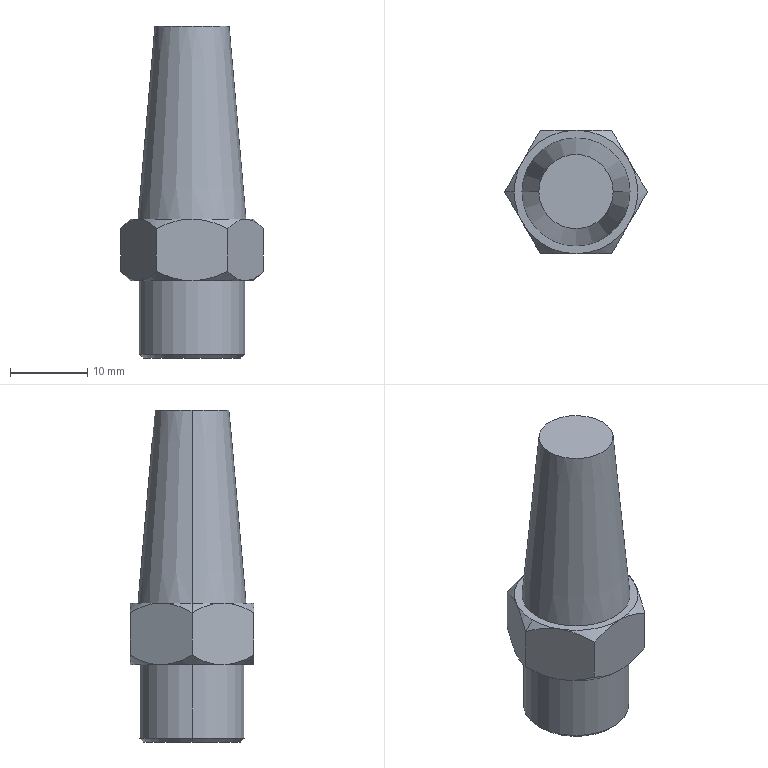Part | SolidWorks | features BaseBody 1 | 1 solid | 33 faces | box 18.475 x 16 x 43 mm | volume 4994 mm3 | cone 18 | plane 11 | cylinder 4 | commonest cylinder face diameters 11.25 x2 13.65 x2
STEP:
#1=CARTESIAN_POINT('',(-4.813,0.,43.));
#2=VERTEX_POINT('',#1);
#3=CARTESIAN_POINT('',(4.813,0.,43.));
#4=VERTEX_POINT('',#3);
#5=CARTESIAN_POINT('',(0.,0.,43.));
#6=DIRECTION('',(0.,0.,-1.));
#7=DIRECTION('',(-1.,0.,0.));
#8=AXIS2_PLACEMENT_3D('',#5,#6,#7);
#9=CIRCLE('',#8,4.813);
#10=EDGE_CURVE('',#2,#4,#9,.T.);
#11=ORIENTED_EDGE('',*,*,#10,.T.);
#12=CARTESIAN_POINT('',(7.,0.,18.));
#13=VERTEX_POINT('',#12);
#14=CARTESIAN_POINT('',(7.,0.,18.));
#15=DIRECTION('',(0.08716,0.,-0.9962));
#16=VECTOR('',#15,1000.);
#17=LINE('',#14,#16);
#18=EDGE_CURVE('',#4,#13,#17,.T.);
#19=ORIENTED_EDGE('',*,*,#18,.T.);
#20=CARTESIAN_POINT('',(-7.,0.,18.));
#21=VERTEX_POINT('',#20);
#22=CARTESIAN_POINT('',(0.,0.,18.));
#23=DIRECTION('',(0.,0.,1.));
#24=DIRECTION('',(-1.,0.,0.));
#25=AXIS2_PLACEMENT_3D('',#22,#23,#24);
#26=CIRCLE('',#25,7.);
#27=EDGE_CURVE('',#13,#21,#26,.T.);
#28=ORIENTED_EDGE('',*,*,#27,.T.);
#29=CARTESIAN_POINT('',(-7.,0.,18.));
#30=DIRECTION('',(-0.08716,0.,-0.9962));
#31=VECTOR('',#30,1000.);
#32=LINE('',#29,#31);
#33=EDGE_CURVE('',#2,#21,#32,.T.);
#34=ORIENTED_EDGE('',*,*,#33,.F.);
#35=EDGE_LOOP('',(#11,#19,#28,#34));
#36=FACE_OUTER_BOUND('',#35,.T.);
#37=CARTESIAN_POINT('',(0.,0.,18.));
#38=DIRECTION('',(0.,0.,-1.));
#39=DIRECTION('',(-1.,0.,0.));
#40=AXIS2_PLACEMENT_3D('',#37,#38,#39);
#41=CONICAL_SURFACE('',#40,7.,0.08727);
#42=ADVANCED_FACE('',(#36),#41,.T.);
#43=CARTESIAN_POINT('',(-8.,0.,18.));
#44=VERTEX_POINT('',#43);
#45=CARTESIAN_POINT('',(-6.928,-4.,18.));
#46=VERTEX_POINT('',#45);
#47=CARTESIAN_POINT('',(0.,0.,18.));
#48=DIRECTION('',(0.,0.,1.));
#49=DIRECTION('',(-1.,0.,0.));
#50=AXIS2_PLACEMENT_3D('',#47,#48,#49);
#51=CIRCLE('',#50,8.);
#52=EDGE_CURVE('',#44,#46,#51,.T.);
#53=ORIENTED_EDGE('',*,*,#52,.F.);
#54=CARTESIAN_POINT('',(-9.238,0.,16.762));
#55=VERTEX_POINT('',#54);
#56=CARTESIAN_POINT('',(-9.245,0.,16.755));
#57=DIRECTION('',(-0.7071,0.,-0.7071));
#58=VECTOR('',#57,1000.);
#59=LINE('',#56,#58);
#60=EDGE_CURVE('',#44,#55,#59,.T.);
#61=ORIENTED_EDGE('',*,*,#60,.T.);
#62=CARTESIAN_POINT('',(-9.238,0.,16.762));
#63=CARTESIAN_POINT('',(-8.876,-0.6269,17.124));
#64=CARTESIAN_POINT('',(-8.506,-1.268,17.432));
#65=CARTESIAN_POINT('',(-7.93,-2.264,17.761));
#66=CARTESIAN_POINT('',(-7.735,-2.602,17.848));
#67=CARTESIAN_POINT('',(-7.337,-3.292,17.968));
#68=CARTESIAN_POINT('',(-7.133,-3.646,18.));
#69=CARTESIAN_POINT('',(-6.928,-4.,18.));
#70=B_SPLINE_CURVE_WITH_KNOTS('',3,(#62,#63,#64,#65,#66,#67,#68,#69),.UNSPECIFIED.,.F.,.F.,(4,2,2,4),(0.,0.002392,0.003589,0.004785),.UNSPECIFIED.);
#71=EDGE_CURVE('',#55,#46,#70,.T.);
#72=ORIENTED_EDGE('',*,*,#71,.T.);
#73=EDGE_LOOP('',(#53,#61,#72));
#74=FACE_OUTER_BOUND('',#73,.T.);
#75=CARTESIAN_POINT('',(0.,0.,16.755));
#76=DIRECTION('',(0.,0.,-1.));
#77=DIRECTION('',(-1.,0.,0.));
#78=AXIS2_PLACEMENT_3D('',#75,#76,#77);
#79=CONICAL_SURFACE('',#78,9.245,0.7854);
#80=ADVANCED_FACE('',(#74),#79,.T.);
#81=CARTESIAN_POINT('',(6.928,-4.,10.));
#82=VERTEX_POINT('',#81);
#83=CARTESIAN_POINT('',(8.,0.,10.));
#84=VERTEX_POINT('',#83);
#85=CARTESIAN_POINT('',(0.,0.,10.));
#86=DIRECTION('',(0.,0.,1.));
#87=DIRECTION('',(1.,0.,0.));
#88=AXIS2_PLACEMENT_3D('',#85,#86,#87);
#89=CIRCLE('',#88,8.);
#90=EDGE_CURVE('',#82,#84,#89,.T.);
#91=ORIENTED_EDGE('',*,*,#90,.T.);
#92=CARTESIAN_POINT('',(9.238,0.,11.238));
#93=VERTEX_POINT('',#92);
#94=CARTESIAN_POINT('',(9.245,0.,11.245));
#95=DIRECTION('',(0.7071,0.,0.7071));
#96=VECTOR('',#95,1000.);
#97=LINE('',#94,#96);
#98=EDGE_CURVE('',#84,#93,#97,.T.);
#99=ORIENTED_EDGE('',*,*,#98,.T.);
#100=CARTESIAN_POINT('',(6.928,-4.,10.));
#101=CARTESIAN_POINT('',(7.334,-3.298,10.));
#102=CARTESIAN_POINT('',(7.728,-2.614,10.125));
#103=CARTESIAN_POINT('',(8.308,-1.61,10.454));
#104=CARTESIAN_POINT('',(8.499,-1.279,10.588));
#105=CARTESIAN_POINT('',(8.874,-0.6306,10.889));
#106=CARTESIAN_POINT('',(9.057,-0.3129,11.057));
#107=CARTESIAN_POINT('',(9.238,0.,11.238));
#108=B_SPLINE_CURVE_WITH_KNOTS('',3,(#100,#101,#102,#103,#104,#105,#106,#107),.UNSPECIFIED.,.F.,.F.,(4,2,2,4),(0.,0.002397,0.003596,0.004794),.UNSPECIFIED.);
#109=EDGE_CURVE('',#82,#93,#108,.T.);
#110=ORIENTED_EDGE('',*,*,#109,.F.);
#111=EDGE_LOOP('',(#91,#99,#110));
#112=FACE_OUTER_BOUND('',#111,.T.);
#113=CARTESIAN_POINT('',(0.,0.,11.245));
#114=DIRECTION('',(0.,0.,1.));
#115=DIRECTION('',(1.,0.,0.));
#116=AXIS2_PLACEMENT_3D('',#113,#114,#115);
#117=CONICAL_SURFACE('',#116,9.245,0.7854);
#118=ADVANCED_FACE('',(#112),#117,.T.);
#119=CARTESIAN_POINT('',(-6.825,0.,10.));
#120=VERTEX_POINT('',#119);
#121=CARTESIAN_POINT('',(6.825,0.,10.));
#122=VERTEX_POINT('',#121);
#123=CARTESIAN_POINT('',(0.,0.,10.));
#124=DIRECTION('',(0.,0.,-1.));
#125=DIRECTION('',(-1.,0.,0.));
#126=AXIS2_PLACEMENT_3D('',#123,#124,#125);
#127=CIRCLE('',#126,6.825);
#128=EDGE_CURVE('',#120,#122,#127,.T.);
#129=ORIENTED_EDGE('',*,*,#128,.T.);
#130=CARTESIAN_POINT('',(6.825,0.,0.5));
#131=VERTEX_POINT('',#130);
#132=CARTESIAN_POINT('',(6.825,0.,10.));
#133=DIRECTION('',(0.,0.,-1.));
#134=VECTOR('',#133,1000.);
#135=LINE('',#132,#134);
#136=EDGE_CURVE('',#122,#131,#135,.T.);
#137=ORIENTED_EDGE('',*,*,#136,.T.);
#138=CARTESIAN_POINT('',(-6.825,0.,0.5));
#139=VERTEX_POINT('',#138);
#140=CARTESIAN_POINT('',(0.,0.,0.5));
#141=DIRECTION('',(0.,0.,1.));
#142=DIRECTION('',(-1.,0.,0.));
#143=AXIS2_PLACEMENT_3D('',#140,#141,#142);
#144=CIRCLE('',#143,6.825);
#145=EDGE_CURVE('',#131,#139,#144,.T.);
#146=ORIENTED_EDGE('',*,*,#145,.T.);
#147=CARTESIAN_POINT('',(-6.825,0.,10.));
#148=DIRECTION('',(0.,0.,-1.));
#149=VECTOR('',#148,1000.);
#150=LINE('',#147,#149);
#151=EDGE_CURVE('',#120,#139,#150,.T.);
#152=ORIENTED_EDGE('',*,*,#151,.F.);
#153=EDGE_LOOP('',(#129,#137,#146,#152));
#154=FACE_OUTER_BOUND('',#153,.T.);
#155=CARTESIAN_POINT('',(0.,0.,10.));
#156=DIRECTION('',(0.,0.,-1.));
#157=DIRECTION('',(-1.,0.,0.));
#158=AXIS2_PLACEMENT_3D('',#155,#156,#157);
#159=CYLINDRICAL_SURFACE('',#158,6.825);
#160=ADVANCED_FACE('',(#154),#159,.T.);
#161=CARTESIAN_POINT('',(6.325,0.,0.));
#162=VERTEX_POINT('',#161);
#163=CARTESIAN_POINT('',(-6.325,0.,0.));
#164=VERTEX_POINT('',#163);
#165=CARTESIAN_POINT('',(0.,0.,0.));
#166=DIRECTION('',(0.,0.,1.));
#167=DIRECTION('',(1.,0.,0.));
#168=AXIS2_PLACEMENT_3D('',#165,#166,#167);
#169=CIRCLE('',#168,6.325);
#170=EDGE_CURVE('',#162,#164,#169,.T.);
#171=ORIENTED_EDGE('',*,*,#170,.T.);
#172=CARTESIAN_POINT('',(-6.825,0.,0.5));
#173=DIRECTION('',(-0.7071,0.,0.7071));
#174=VECTOR('',#173,1000.);
#175=LINE('',#172,#174);
#176=EDGE_CURVE('',#164,#139,#175,.T.);
#177=ORIENTED_EDGE('',*,*,#176,.T.);
#178=ORIENTED_EDGE('',*,*,#145,.F.);
#179=CARTESIAN_POINT('',(6.825,0.,0.5));
#180=DIRECTION('',(0.7071,0.,0.7071));
#181=VECTOR('',#180,1000.);
#182=LINE('',#179,#181);
#183=EDGE_CURVE('',#162,#131,#182,.T.);
#184=ORIENTED_EDGE('',*,*,#183,.F.);
#185=EDGE_LOOP('',(#171,#177,#178,#184));
#186=FACE_OUTER_BOUND('',#185,.T.);
#187=CARTESIAN_POINT('',(0.,0.,0.5));
#188=DIRECTION('',(0.,0.,1.));
#189=DIRECTION('',(1.,0.,0.));
#190=AXIS2_PLACEMENT_3D('',#187,#188,#189);
#191=CONICAL_SURFACE('',#190,6.825,0.7854);
#192=ADVANCED_FACE('',(#186),#191,.T.);
#193=CARTESIAN_POINT('',(5.625,0.,10.));
#194=VERTEX_POINT('',#193);
#195=CARTESIAN_POINT('',(-5.625,0.,10.));
#196=VERTEX_POINT('',#195);
#197=CARTESIAN_POINT('',(0.,0.,10.));
#198=DIRECTION('',(0.,0.,-1.));
#199=DIRECTION('',(-1.,0.,0.));
#200=AXIS2_PLACEMENT_3D('',#197,#198,#199);
#201=CIRCLE('',#200,5.625);
#202=EDGE_CURVE('',#194,#196,#201,.T.);
#203=ORIENTED_EDGE('',*,*,#202,.F.);
#204=CARTESIAN_POINT('',(5.625,0.,0.));
#205=VERTEX_POINT('',#204);
#206=CARTESIAN_POINT('',(5.625,0.,10.));
#207=DIRECTION('',(0.,0.,-1.));
#208=VECTOR('',#207,1000.);
#209=LINE('',#206,#208);
#210=EDGE_CURVE('',#194,#205,#209,.T.);
#211=ORIENTED_EDGE('',*,*,#210,.T.);
#212=CARTESIAN_POINT('',(-5.625,0.,0.));
#213=VERTEX_POINT('',#212);
#214=CARTESIAN_POINT('',(0.,0.,0.));
#215=DIRECTION('',(0.,0.,-1.));
#216=DIRECTION('',(-1.,0.,0.));
#217=AXIS2_PLACEMENT_3D('',#214,#215,#216);
#218=CIRCLE('',#217,5.625);
#219=EDGE_CURVE('',#205,#213,#218,.T.);
#220=ORIENTED_EDGE('',*,*,#219,.T.);
#221=CARTESIAN_POINT('',(-5.625,0.,10.));
#222=DIRECTION('',(0.,0.,-1.));
#223=VECTOR('',#222,1000.);
#224=LINE('',#221,#223);
#225=EDGE_CURVE('',#196,#213,#224,.T.);
#226=ORIENTED_EDGE('',*,*,#225,.F.);
#227=EDGE_LOOP('',(#203,#211,#220,#226));
#228=FACE_OUTER_BOUND('',#227,.T.);
#229=CARTESIAN_POINT('',(0.,0.,10.));
#230=DIRECTION('',(0.,0.,-1.));
#231=DIRECTION('',(-1.,0.,0.));
#232=AXIS2_PLACEMENT_3D('',#229,#230,#231);
#233=CYLINDRICAL_SURFACE('',#232,5.625);
#234=ADVANCED_FACE('',(#228),#233,.F.);
#235=ORIENTED_EDGE('',*,*,#18,.F.);
#236=CARTESIAN_POINT('',(0.,0.,43.));
#237=DIRECTION('',(0.,0.,-1.));
#238=DIRECTION('',(-1.,0.,0.));
#239=AXIS2_PLACEMENT_3D('',#236,#237,#238);
#240=CIRCLE('',#239,4.813);
#241=EDGE_CURVE('',#4,#2,#240,.T.);
#242=ORIENTED_EDGE('',*,*,#241,.T.);
#243=ORIENTED_EDGE('',*,*,#33,.T.);
#244=CARTESIAN_POINT('',(0.,0.,18.));
#245=DIRECTION('',(0.,0.,1.));
#246=DIRECTION('',(-1.,0.,0.));
#247=AXIS2_PLACEMENT_3D('',#244,#245,#246);
#248=CIRCLE('',#247,7.);
#249=EDGE_CURVE('',#21,#13,#248,.T.);
#250=ORIENTED_EDGE('',*,*,#249,.T.);
#251=EDGE_LOOP('',(#235,#242,#243,#250));
#252=FACE_OUTER_BOUND('',#251,.T.);
#253=CARTESIAN_POINT('',(0.,0.,18.));
#254=DIRECTION('',(0.,0.,-1.));
#255=DIRECTION('',(-1.,0.,0.));
#256=AXIS2_PLACEMENT_3D('',#253,#254,#255);
#257=CONICAL_SURFACE('',#256,7.,0.08727);
#258=ADVANCED_FACE('',(#252),#257,.T.);
#259=ORIENTED_EDGE('',*,*,#249,.F.);
#260=ORIENTED_EDGE('',*,*,#27,.F.);
#261=EDGE_LOOP('',(#259,#260));
#262=FACE_BOUND('',#261,.T.);
#263=CARTESIAN_POINT('',(0.,-8.,18.));
#264=VERTEX_POINT('',#263);
#265=CARTESIAN_POINT('',(6.928,-4.,18.));
#266=VERTEX_POINT('',#265);
#267=CARTESIAN_POINT('',(0.,0.,18.));
#268=DIRECTION('',(0.,0.,1.));
#269=DIRECTION('',(-1.,0.,0.));
#270=AXIS2_PLACEMENT_3D('',#267,#268,#269);
#271=CIRCLE('',#270,8.);
#272=EDGE_CURVE('',#264,#266,#271,.T.);
#273=ORIENTED_EDGE('',*,*,#272,.T.);
#274=CARTESIAN_POINT('',(6.928,4.,18.));
#275=VERTEX_POINT('',#274);
#276=CARTESIAN_POINT('',(0.,0.,18.));
#277=DIRECTION('',(0.,0.,1.));
#278=DIRECTION('',(-1.,0.,0.));
#279=AXIS2_PLACEMENT_3D('',#276,#277,#278);
#280=CIRCLE('',#279,8.);
#281=EDGE_CURVE('',#266,#275,#280,.T.);
#282=ORIENTED_EDGE('',*,*,#281,.T.);
#283=CARTESIAN_POINT('',(0.,8.,18.));
#284=VERTEX_POINT('',#283);
#285=CARTESIAN_POINT('',(0.,0.,18.));
#286=DIRECTION('',(0.,0.,1.));
#287=DIRECTION('',(-1.,0.,0.));
#288=AXIS2_PLACEMENT_3D('',#285,#286,#287);
#289=CIRCLE('',#288,8.);
#290=EDGE_CURVE('',#275,#284,#289,.T.);
#291=ORIENTED_EDGE('',*,*,#290,.T.);
#292=CARTESIAN_POINT('',(-6.928,4.,18.));
#293=VERTEX_POINT('',#292);
#294=CARTESIAN_POINT('',(0.,0.,18.));
#295=DIRECTION('',(0.,0.,1.));
#296=DIRECTION('',(-1.,0.,0.));
#297=AXIS2_PLACEMENT_3D('',#294,#295,#296);
#298=CIRCLE('',#297,8.);
#299=EDGE_CURVE('',#284,#293,#298,.T.);
#300=ORIENTED_EDGE('',*,*,#299,.T.);
#301=CARTESIAN_POINT('',(0.,0.,18.));
#302=DIRECTION('',(0.,0.,1.));
#303=DIRECTION('',(-1.,0.,0.));
#304=AXIS2_PLACEMENT_3D('',#301,#302,#303);
#305=CIRCLE('',#304,8.);
#306=EDGE_CURVE('',#293,#44,#305,.T.);
#307=ORIENTED_EDGE('',*,*,#306,.T.);
#308=ORIENTED_EDGE('',*,*,#52,.T.);
#309=CARTESIAN_POINT('',(0.,0.,18.));
#310=DIRECTION('',(0.,0.,1.));
#311=DIRECTION('',(-1.,0.,0.));
#312=AXIS2_PLACEMENT_3D('',#309,#310,#311);
#313=CIRCLE('',#312,8.);
#314=EDGE_CURVE('',#46,#264,#313,.T.);
#315=ORIENTED_EDGE('',*,*,#314,.T.);
#316=EDGE_LOOP('',(#273,#282,#291,#300,#307,#308,#315));
#317=FACE_OUTER_BOUND('',#316,.T.);
#318=CARTESIAN_POINT('',(0.,0.,18.));
#319=DIRECTION('',(0.,0.,1.));
#320=DIRECTION('',(1.,0.,0.));
#321=AXIS2_PLACEMENT_3D('',#318,#319,#320);
#322=PLANE('',#321);
#323=ADVANCED_FACE('',(#262,#317),#322,.T.);
#324=ORIENTED_EDGE('',*,*,#10,.F.);
#325=ORIENTED_EDGE('',*,*,#241,.F.);
#326=EDGE_LOOP('',(#324,#325));
#327=FACE_OUTER_BOUND('',#326,.T.);
#328=CARTESIAN_POINT('',(0.,0.,43.));
#329=DIRECTION('',(0.,0.,1.));
#330=DIRECTION('',(1.,0.,0.));
#331=AXIS2_PLACEMENT_3D('',#328,#329,#330);
#332=PLANE('',#331);
#333=ADVANCED_FACE('',(#327),#332,.T.);
#334=CARTESIAN_POINT('',(9.238,-0.000000006,16.762));
#335=VERTEX_POINT('',#334);
#336=CARTESIAN_POINT('',(6.928,-4.,18.));
#337=CARTESIAN_POINT('',(7.334,-3.298,18.));
#338=CARTESIAN_POINT('',(7.728,-2.614,17.875));
#339=CARTESIAN_POINT('',(8.308,-1.61,17.546));
#340=CARTESIAN_POINT('',(8.499,-1.279,17.412));
#341=CARTESIAN_POINT('',(8.874,-0.6306,17.111));
#342=CARTESIAN_POINT('',(9.057,-0.3129,16.943));
#343=CARTESIAN_POINT('',(9.238,-0.000000006,16.762));
#344=B_SPLINE_CURVE_WITH_KNOTS('',3,(#336,#337,#338,#339,#340,#341,#342,#343),.UNSPECIFIED.,.F.,.F.,(4,2,2,4),(0.,0.002397,0.003596,0.004794),.UNSPECIFIED.);
#345=EDGE_CURVE('',#266,#335,#344,.T.);
#346=ORIENTED_EDGE('',*,*,#345,.T.);
#347=CARTESIAN_POINT('',(9.238,-0.000000006,16.762));
#348=CARTESIAN_POINT('',(8.876,0.6269,17.124));
#349=CARTESIAN_POINT('',(8.506,1.268,17.432));
#350=CARTESIAN_POINT('',(7.93,2.264,17.761));
#351=CARTESIAN_POINT('',(7.735,2.602,17.848));
#352=CARTESIAN_POINT('',(7.337,3.292,17.968));
#353=CARTESIAN_POINT('',(7.133,3.646,18.));
#354=CARTESIAN_POINT('',(6.928,4.,18.));
#355=B_SPLINE_CURVE_WITH_KNOTS('',3,(#347,#348,#349,#350,#351,#352,#353,#354),.UNSPECIFIED.,.F.,.F.,(4,2,2,4),(0.,0.002392,0.003589,0.004785),.UNSPECIFIED.);
#356=EDGE_CURVE('',#335,#275,#355,.T.);
#357=ORIENTED_EDGE('',*,*,#356,.T.);
#358=ORIENTED_EDGE('',*,*,#281,.F.);
#359=EDGE_LOOP('',(#346,#357,#358));
#360=FACE_OUTER_BOUND('',#359,.T.);
#361=CARTESIAN_POINT('',(0.,0.,16.755));
#362=DIRECTION('',(0.,0.,-1.));
#363=DIRECTION('',(-1.,0.,0.));
#364=AXIS2_PLACEMENT_3D('',#361,#362,#363);
#365=CONICAL_SURFACE('',#364,9.245,0.7854);
#366=ADVANCED_FACE('',(#360),#365,.T.);
#367=CARTESIAN_POINT('',(4.619,-8.,16.762));
#368=VERTEX_POINT('',#367);
#369=CARTESIAN_POINT('',(0.,-8.,18.));
#370=CARTESIAN_POINT('',(0.811,-8.,18.));
#371=CARTESIAN_POINT('',(1.6,-8.,17.875));
#372=CARTESIAN_POINT('',(2.76,-8.,17.546));
#373=CARTESIAN_POINT('',(3.142,-8.,17.412));
#374=CARTESIAN_POINT('',(3.891,-8.,17.111));
#375=CARTESIAN_POINT('',(4.257,-8.,16.943));
#376=CARTESIAN_POINT('',(4.619,-8.,16.762));
#377=B_SPLINE_CURVE_WITH_KNOTS('',3,(#369,#370,#371,#372,#373,#374,#375,#376),.UNSPECIFIED.,.F.,.F.,(4,2,2,4),(0.,0.002397,0.003596,0.004794),.UNSPECIFIED.);
#378=EDGE_CURVE('',#264,#368,#377,.T.);
#379=ORIENTED_EDGE('',*,*,#378,.T.);
#380=CARTESIAN_POINT('',(4.619,-8.,16.762));
#381=CARTESIAN_POINT('',(4.981,-7.373,17.124));
#382=CARTESIAN_POINT('',(5.351,-6.732,17.432));
#383=CARTESIAN_POINT('',(5.926,-5.736,17.761));
#384=CARTESIAN_POINT('',(6.121,-5.398,17.848));
#385=CARTESIAN_POINT('',(6.519,-4.708,17.968));
#386=CARTESIAN_POINT('',(6.724,-4.354,18.));
#387=CARTESIAN_POINT('',(6.928,-4.,18.));
#388=B_SPLINE_CURVE_WITH_KNOTS('',3,(#380,#381,#382,#383,#384,#385,#386,#387),.UNSPECIFIED.,.F.,.F.,(4,2,2,4),(0.,0.002392,0.003589,0.004785),.UNSPECIFIED.);
#389=EDGE_CURVE('',#368,#266,#388,.T.);
#390=ORIENTED_EDGE('',*,*,#389,.T.);
#391=ORIENTED_EDGE('',*,*,#272,.F.);
#392=EDGE_LOOP('',(#379,#390,#391));
#393=FACE_OUTER_BOUND('',#392,.T.);
#394=CARTESIAN_POINT('',(0.,0.,16.755));
#395=DIRECTION('',(0.,0.,-1.));
#396=DIRECTION('',(-1.,0.,0.));
#397=AXIS2_PLACEMENT_3D('',#394,#395,#396);
#398=CONICAL_SURFACE('',#397,9.245,0.7854);
#399=ADVANCED_FACE('',(#393),#398,.T.);
#400=CARTESIAN_POINT('',(-4.619,-8.,16.762));
#401=VERTEX_POINT('',#400);
#402=CARTESIAN_POINT('',(-6.928,-4.,18.));
#403=CARTESIAN_POINT('',(-6.523,-4.702,18.));
#404=CARTESIAN_POINT('',(-6.128,-5.386,17.875));
#405=CARTESIAN_POINT('',(-5.548,-6.39,17.546));
#406=CARTESIAN_POINT('',(-5.357,-6.721,17.412));
#407=CARTESIAN_POINT('',(-4.983,-7.369,17.111));
#408=CARTESIAN_POINT('',(-4.799,-7.687,16.943));
#409=CARTESIAN_POINT('',(-4.619,-8.,16.762));
#410=B_SPLINE_CURVE_WITH_KNOTS('',3,(#402,#403,#404,#405,#406,#407,#408,#409),.UNSPECIFIED.,.F.,.F.,(4,2,2,4),(0.,0.002397,0.003596,0.004794),.UNSPECIFIED.);
#411=EDGE_CURVE('',#46,#401,#410,.T.);
#412=ORIENTED_EDGE('',*,*,#411,.T.);
#413=CARTESIAN_POINT('',(-4.619,-8.,16.762));
#414=CARTESIAN_POINT('',(-3.895,-8.,17.124));
#415=CARTESIAN_POINT('',(-3.155,-8.,17.432));
#416=CARTESIAN_POINT('',(-2.005,-8.,17.761));
#417=CARTESIAN_POINT('',(-1.614,-8.,17.848));
#418=CARTESIAN_POINT('',(-0.8177,-8.,17.968));
#419=CARTESIAN_POINT('',(-0.4086,-8.,18.));
#420=CARTESIAN_POINT('',(0.,-8.,18.));
#421=B_SPLINE_CURVE_WITH_KNOTS('',3,(#413,#414,#415,#416,#417,#418,#419,#420),.UNSPECIFIED.,.F.,.F.,(4,2,2,4),(0.,0.002392,0.003589,0.004785),.UNSPECIFIED.);
#422=EDGE_CURVE('',#401,#264,#421,.T.);
#423=ORIENTED_EDGE('',*,*,#422,.T.);
#424=ORIENTED_EDGE('',*,*,#314,.F.);
#425=EDGE_LOOP('',(#412,#423,#424));
#426=FACE_OUTER_BOUND('',#425,.T.);
#427=CARTESIAN_POINT('',(0.,0.,16.755));
#428=DIRECTION('',(0.,0.,-1.));
#429=DIRECTION('',(-1.,0.,0.));
#430=AXIS2_PLACEMENT_3D('',#427,#428,#429);
#431=CONICAL_SURFACE('',#430,9.245,0.7854);
#432=ADVANCED_FACE('',(#426),#431,.T.);
#433=ORIENTED_EDGE('',*,*,#60,.F.);
#434=ORIENTED_EDGE('',*,*,#306,.F.);
#435=CARTESIAN_POINT('',(-6.928,4.,18.));
#436=CARTESIAN_POINT('',(-7.334,3.298,18.));
#437=CARTESIAN_POINT('',(-7.728,2.614,17.875));
#438=CARTESIAN_POINT('',(-8.308,1.61,17.546));
#439=CARTESIAN_POINT('',(-8.499,1.279,17.412));
#440=CARTESIAN_POINT('',(-8.874,0.6306,17.111));
#441=CARTESIAN_POINT('',(-9.057,0.3129,16.943));
#442=CARTESIAN_POINT('',(-9.238,0.,16.762));
#443=B_SPLINE_CURVE_WITH_KNOTS('',3,(#435,#436,#437,#438,#439,#440,#441,#442),.UNSPECIFIED.,.F.,.F.,(4,2,2,4),(0.,0.002397,0.003596,0.004794),.UNSPECIFIED.);
#444=EDGE_CURVE('',#293,#55,#443,.T.);
#445=ORIENTED_EDGE('',*,*,#444,.T.);
#446=EDGE_LOOP('',(#433,#434,#445));
#447=FACE_OUTER_BOUND('',#446,.T.);
#448=CARTESIAN_POINT('',(0.,0.,16.755));
#449=DIRECTION('',(0.,0.,-1.));
#450=DIRECTION('',(-1.,0.,0.));
#451=AXIS2_PLACEMENT_3D('',#448,#449,#450);
#452=CONICAL_SURFACE('',#451,9.245,0.7854);
#453=ADVANCED_FACE('',(#447),#452,.T.);
#454=CARTESIAN_POINT('',(-4.619,8.,16.762));
#455=VERTEX_POINT('',#454);
#456=CARTESIAN_POINT('',(-4.619,8.,16.762));
#457=CARTESIAN_POINT('',(-4.981,7.373,17.124));
#458=CARTESIAN_POINT('',(-5.351,6.732,17.432));
#459=CARTESIAN_POINT('',(-5.926,5.736,17.761));
#460=CARTESIAN_POINT('',(-6.121,5.398,17.848));
#461=CARTESIAN_POINT('',(-6.519,4.708,17.968));
#462=CARTESIAN_POINT('',(-6.724,4.354,18.));
#463=CARTESIAN_POINT('',(-6.928,4.,18.));
#464=B_SPLINE_CURVE_WITH_KNOTS('',3,(#456,#457,#458,#459,#460,#461,#462,#463),.UNSPECIFIED.,.F.,.F.,(4,2,2,4),(0.,0.002392,0.003589,0.004785),.UNSPECIFIED.);
#465=EDGE_CURVE('',#455,#293,#464,.T.);
#466=ORIENTED_EDGE('',*,*,#465,.T.);
#467=ORIENTED_EDGE('',*,*,#299,.F.);
#468=CARTESIAN_POINT('',(0.,8.,18.));
#469=CARTESIAN_POINT('',(-0.811,8.,18.));
#470=CARTESIAN_POINT('',(-1.6,8.,17.875));
#471=CARTESIAN_POINT('',(-2.76,8.,17.546));
#472=CARTESIAN_POINT('',(-3.142,8.,17.412));
#473=CARTESIAN_POINT('',(-3.891,8.,17.111));
#474=CARTESIAN_POINT('',(-4.257,8.,16.943));
#475=CARTESIAN_POINT('',(-4.619,8.,16.762));
#476=B_SPLINE_CURVE_WITH_KNOTS('',3,(#468,#469,#470,#471,#472,#473,#474,#475),.UNSPECIFIED.,.F.,.F.,(4,2,2,4),(0.,0.002397,0.003596,0.004794),.UNSPECIFIED.);
#477=EDGE_CURVE('',#284,#455,#476,.T.);
#478=ORIENTED_EDGE('',*,*,#477,.T.);
#479=EDGE_LOOP('',(#466,#467,#478));
#480=FACE_OUTER_BOUND('',#479,.T.);
#481=CARTESIAN_POINT('',(0.,0.,16.755));
#482=DIRECTION('',(0.,0.,-1.));
#483=DIRECTION('',(-1.,0.,0.));
#484=AXIS2_PLACEMENT_3D('',#481,#482,#483);
#485=CONICAL_SURFACE('',#484,9.245,0.7854);
#486=ADVANCED_FACE('',(#480),#485,.T.);
#487=CARTESIAN_POINT('',(4.619,8.,16.762));
#488=VERTEX_POINT('',#487);
#489=CARTESIAN_POINT('',(4.619,8.,16.762));
#490=CARTESIAN_POINT('',(3.895,8.,17.124));
#491=CARTESIAN_POINT('',(3.155,8.,17.432));
#492=CARTESIAN_POINT('',(2.005,8.,17.761));
#493=CARTESIAN_POINT('',(1.614,8.,17.848));
#494=CARTESIAN_POINT('',(0.8177,8.,17.968));
#495=CARTESIAN_POINT('',(0.4086,8.,18.));
#496=CARTESIAN_POINT('',(0.,8.,18.));
#497=B_SPLINE_CURVE_WITH_KNOTS('',3,(#489,#490,#491,#492,#493,#494,#495,#496),.UNSPECIFIED.,.F.,.F.,(4,2,2,4),(0.,0.002392,0.003589,0.004785),.UNSPECIFIED.);
#498=EDGE_CURVE('',#488,#284,#497,.T.);
#499=ORIENTED_EDGE('',*,*,#498,.T.);
#500=ORIENTED_EDGE('',*,*,#290,.F.);
#501=CARTESIAN_POINT('',(6.928,4.,18.));
#502=CARTESIAN_POINT('',(6.523,4.702,18.));
#503=CARTESIAN_POINT('',(6.128,5.386,17.875));
#504=CARTESIAN_POINT('',(5.548,6.39,17.546));
#505=CARTESIAN_POINT('',(5.357,6.721,17.412));
#506=CARTESIAN_POINT('',(4.983,7.369,17.111));
#507=CARTESIAN_POINT('',(4.799,7.687,16.943));
#508=CARTESIAN_POINT('',(4.619,8.,16.762));
#509=B_SPLINE_CURVE_WITH_KNOTS('',3,(#501,#502,#503,#504,#505,#506,#507,#508),.UNSPECIFIED.,.F.,.F.,(4,2,2,4),(0.,0.002397,0.003596,0.004794),.UNSPECIFIED.);
#510=EDGE_CURVE('',#275,#488,#509,.T.);
#511=ORIENTED_EDGE('',*,*,#510,.T.);
#512=EDGE_LOOP('',(#499,#500,#511));
#513=FACE_OUTER_BOUND('',#512,.T.);
#514=CARTESIAN_POINT('',(0.,0.,16.755));
#515=DIRECTION('',(0.,0.,-1.));
#516=DIRECTION('',(-1.,0.,0.));
#517=AXIS2_PLACEMENT_3D('',#514,#515,#516);
#518=CONICAL_SURFACE('',#517,9.245,0.7854);
#519=ADVANCED_FACE('',(#513),#518,.T.);
#520=CARTESIAN_POINT('',(6.928,4.,10.));
#521=VERTEX_POINT('',#520);
#522=CARTESIAN_POINT('',(9.238,0.,11.238));
#523=CARTESIAN_POINT('',(8.876,0.6269,10.876));
#524=CARTESIAN_POINT('',(8.506,1.268,10.568));
#525=CARTESIAN_POINT('',(7.93,2.264,10.239));
#526=CARTESIAN_POINT('',(7.735,2.602,10.152));
#527=CARTESIAN_POINT('',(7.337,3.292,10.032));
#528=CARTESIAN_POINT('',(7.133,3.646,10.));
#529=CARTESIAN_POINT('',(6.928,4.,10.));
#530=B_SPLINE_CURVE_WITH_KNOTS('',3,(#522,#523,#524,#525,#526,#527,#528,#529),.UNSPECIFIED.,.F.,.F.,(4,2,2,4),(0.,0.002392,0.003589,0.004785),.UNSPECIFIED.);
#531=EDGE_CURVE('',#93,#521,#530,.T.);
#532=ORIENTED_EDGE('',*,*,#531,.T.);
#533=CARTESIAN_POINT('',(4.619,8.,11.238));
#534=VERTEX_POINT('',#533);
#535=CARTESIAN_POINT('',(6.928,4.,10.));
#536=CARTESIAN_POINT('',(6.523,4.702,10.));
#537=CARTESIAN_POINT('',(6.128,5.386,10.125));
#538=CARTESIAN_POINT('',(5.548,6.39,10.454));
#539=CARTESIAN_POINT('',(5.357,6.721,10.588));
#540=CARTESIAN_POINT('',(4.983,7.369,10.889));
#541=CARTESIAN_POINT('',(4.799,7.687,11.057));
#542=CARTESIAN_POINT('',(4.619,8.,11.238));
#543=B_SPLINE_CURVE_WITH_KNOTS('',3,(#535,#536,#537,#538,#539,#540,#541,#542),.UNSPECIFIED.,.F.,.F.,(4,2,2,4),(0.,0.002397,0.003596,0.004794),.UNSPECIFIED.);
#544=EDGE_CURVE('',#521,#534,#543,.T.);
#545=ORIENTED_EDGE('',*,*,#544,.T.);
#546=CARTESIAN_POINT('',(4.619,8.,10.));
#547=DIRECTION('',(0.,0.,1.));
#548=VECTOR('',#547,1000.);
#549=LINE('',#546,#548);
#550=EDGE_CURVE('',#534,#488,#549,.T.);
#551=ORIENTED_EDGE('',*,*,#550,.T.);
#552=ORIENTED_EDGE('',*,*,#510,.F.);
#553=ORIENTED_EDGE('',*,*,#356,.F.);
#554=CARTESIAN_POINT('',(9.238,0.,10.));
#555=DIRECTION('',(0.,0.,-1.));
#556=VECTOR('',#555,1000.);
#557=LINE('',#554,#556);
#558=EDGE_CURVE('',#335,#93,#557,.T.);
#559=ORIENTED_EDGE('',*,*,#558,.T.);
#560=EDGE_LOOP('',(#532,#545,#551,#552,#553,#559));
#561=FACE_OUTER_BOUND('',#560,.T.);
#562=CARTESIAN_POINT('',(9.238,0.,10.));
#563=DIRECTION('',(0.866,0.5,0.));
#564=DIRECTION('',(-0.5,0.866,0.));
#565=AXIS2_PLACEMENT_3D('',#562,#563,#564);
#566=PLANE('',#565);
#567=ADVANCED_FACE('',(#561),#566,.T.);
#568=CARTESIAN_POINT('',(4.619,-8.,11.238));
#569=VERTEX_POINT('',#568);
#570=CARTESIAN_POINT('',(4.619,-8.,11.238));
#571=CARTESIAN_POINT('',(4.981,-7.373,10.876));
#572=CARTESIAN_POINT('',(5.351,-6.732,10.568));
#573=CARTESIAN_POINT('',(5.926,-5.736,10.239));
#574=CARTESIAN_POINT('',(6.121,-5.398,10.152));
#575=CARTESIAN_POINT('',(6.519,-4.708,10.032));
#576=CARTESIAN_POINT('',(6.724,-4.354,10.));
#577=CARTESIAN_POINT('',(6.928,-4.,10.));
#578=B_SPLINE_CURVE_WITH_KNOTS('',3,(#570,#571,#572,#573,#574,#575,#576,#577),.UNSPECIFIED.,.F.,.F.,(4,2,2,4),(0.,0.002392,0.003589,0.004785),.UNSPECIFIED.);
#579=EDGE_CURVE('',#569,#82,#578,.T.);
#580=ORIENTED_EDGE('',*,*,#579,.T.);
#581=ORIENTED_EDGE('',*,*,#109,.T.);
#582=ORIENTED_EDGE('',*,*,#558,.F.);
#583=ORIENTED_EDGE('',*,*,#345,.F.);
#584=ORIENTED_EDGE('',*,*,#389,.F.);
#585=CARTESIAN_POINT('',(4.619,-8.,10.));
#586=DIRECTION('',(0.,0.,-1.));
#587=VECTOR('',#586,1000.);
#588=LINE('',#585,#587);
#589=EDGE_CURVE('',#368,#569,#588,.T.);
#590=ORIENTED_EDGE('',*,*,#589,.T.);
#591=EDGE_LOOP('',(#580,#581,#582,#583,#584,#590));
#592=FACE_OUTER_BOUND('',#591,.T.);
#593=CARTESIAN_POINT('',(4.619,-8.,10.));
#594=DIRECTION('',(0.866,-0.5,0.));
#595=DIRECTION('',(0.5,0.866,0.));
#596=AXIS2_PLACEMENT_3D('',#593,#594,#595);
#597=PLANE('',#596);
#598=ADVANCED_FACE('',(#592),#597,.T.);
#599=CARTESIAN_POINT('',(-4.619,-8.,11.238));
#600=VERTEX_POINT('',#599);
#601=CARTESIAN_POINT('',(0.,-8.,10.));
#602=VERTEX_POINT('',#601);
#603=CARTESIAN_POINT('',(-4.619,-8.,11.238));
#604=CARTESIAN_POINT('',(-3.895,-8.,10.876));
#605=CARTESIAN_POINT('',(-3.155,-8.,10.568));
#606=CARTESIAN_POINT('',(-2.005,-8.,10.239));
#607=CARTESIAN_POINT('',(-1.614,-8.,10.152));
#608=CARTESIAN_POINT('',(-0.8177,-8.,10.032));
#609=CARTESIAN_POINT('',(-0.4086,-8.,10.));
#610=CARTESIAN_POINT('',(0.,-8.,10.));
#611=B_SPLINE_CURVE_WITH_KNOTS('',3,(#603,#604,#605,#606,#607,#608,#609,#610),.UNSPECIFIED.,.F.,.F.,(4,2,2,4),(0.,0.002392,0.003589,0.004785),.UNSPECIFIED.);
#612=EDGE_CURVE('',#600,#602,#611,.T.);
#613=ORIENTED_EDGE('',*,*,#612,.T.);
#614=CARTESIAN_POINT('',(0.,-8.,10.));
#615=CARTESIAN_POINT('',(0.811,-8.,10.));
#616=CARTESIAN_POINT('',(1.6,-8.,10.125));
#617=CARTESIAN_POINT('',(2.76,-8.,10.454));
#618=CARTESIAN_POINT('',(3.142,-8.,10.588));
#619=CARTESIAN_POINT('',(3.891,-8.,10.889));
#620=CARTESIAN_POINT('',(4.257,-8.,11.057));
#621=CARTESIAN_POINT('',(4.619,-8.,11.238));
#622=B_SPLINE_CURVE_WITH_KNOTS('',3,(#614,#615,#616,#617,#618,#619,#620,#621),.UNSPECIFIED.,.F.,.F.,(4,2,2,4),(0.,0.002397,0.003596,0.004794),.UNSPECIFIED.);
#623=EDGE_CURVE('',#602,#569,#622,.T.);
#624=ORIENTED_EDGE('',*,*,#623,.T.);
#625=ORIENTED_EDGE('',*,*,#589,.F.);
#626=ORIENTED_EDGE('',*,*,#378,.F.);
#627=ORIENTED_EDGE('',*,*,#422,.F.);
#628=CARTESIAN_POINT('',(-4.619,-8.,10.));
#629=DIRECTION('',(0.,0.,-1.));
#630=VECTOR('',#629,1000.);
#631=LINE('',#628,#630);
#632=EDGE_CURVE('',#401,#600,#631,.T.);
#633=ORIENTED_EDGE('',*,*,#632,.T.);
#634=EDGE_LOOP('',(#613,#624,#625,#626,#627,#633));
#635=FACE_OUTER_BOUND('',#634,.T.);
#636=CARTESIAN_POINT('',(-4.619,-8.,10.));
#637=DIRECTION('',(0.,-1.,0.));
#638=DIRECTION('',(1.,0.,0.));
#639=AXIS2_PLACEMENT_3D('',#636,#637,#638);
#640=PLANE('',#639);
#641=ADVANCED_FACE('',(#635),#640,.T.);
#642=CARTESIAN_POINT('',(-9.238,0.,11.238));
#643=VERTEX_POINT('',#642);
#644=CARTESIAN_POINT('',(-6.928,-4.,10.));
#645=VERTEX_POINT('',#644);
#646=CARTESIAN_POINT('',(-9.238,0.,11.238));
#647=CARTESIAN_POINT('',(-8.876,-0.6269,10.876));
#648=CARTESIAN_POINT('',(-8.506,-1.268,10.568));
#649=CARTESIAN_POINT('',(-7.93,-2.264,10.239));
#650=CARTESIAN_POINT('',(-7.735,-2.602,10.152));
#651=CARTESIAN_POINT('',(-7.337,-3.292,10.032));
#652=CARTESIAN_POINT('',(-7.133,-3.646,10.));
#653=CARTESIAN_POINT('',(-6.928,-4.,10.));
#654=B_SPLINE_CURVE_WITH_KNOTS('',3,(#646,#647,#648,#649,#650,#651,#652,#653),.UNSPECIFIED.,.F.,.F.,(4,2,2,4),(0.,0.002392,0.003589,0.004785),.UNSPECIFIED.);
#655=EDGE_CURVE('',#643,#645,#654,.T.);
#656=ORIENTED_EDGE('',*,*,#655,.T.);
#657=CARTESIAN_POINT('',(-6.928,-4.,10.));
#658=CARTESIAN_POINT('',(-6.523,-4.702,10.));
#659=CARTESIAN_POINT('',(-6.128,-5.386,10.125));
#660=CARTESIAN_POINT('',(-5.548,-6.39,10.454));
#661=CARTESIAN_POINT('',(-5.357,-6.721,10.588));
#662=CARTESIAN_POINT('',(-4.983,-7.369,10.889));
#663=CARTESIAN_POINT('',(-4.799,-7.687,11.057));
#664=CARTESIAN_POINT('',(-4.619,-8.,11.238));
#665=B_SPLINE_CURVE_WITH_KNOTS('',3,(#657,#658,#659,#660,#661,#662,#663,#664),.UNSPECIFIED.,.F.,.F.,(4,2,2,4),(0.,0.002397,0.003596,0.004794),.UNSPECIFIED.);
#666=EDGE_CURVE('',#645,#600,#665,.T.);
#667=ORIENTED_EDGE('',*,*,#666,.T.);
#668=ORIENTED_EDGE('',*,*,#632,.F.);
#669=ORIENTED_EDGE('',*,*,#411,.F.);
#670=ORIENTED_EDGE('',*,*,#71,.F.);
#671=CARTESIAN_POINT('',(-9.238,0.,10.));
#672=DIRECTION('',(0.,0.,-1.));
#673=VECTOR('',#672,1000.);
#674=LINE('',#671,#673);
#675=EDGE_CURVE('',#55,#643,#674,.T.);
#676=ORIENTED_EDGE('',*,*,#675,.T.);
#677=EDGE_LOOP('',(#656,#667,#668,#669,#670,#676));
#678=FACE_OUTER_BOUND('',#677,.T.);
#679=CARTESIAN_POINT('',(-9.238,0.,10.));
#680=DIRECTION('',(-0.866,-0.5,0.));
#681=DIRECTION('',(0.5,-0.866,0.));
#682=AXIS2_PLACEMENT_3D('',#679,#680,#681);
#683=PLANE('',#682);
#684=ADVANCED_FACE('',(#678),#683,.T.);
#685=CARTESIAN_POINT('',(-4.619,8.,11.238));
#686=VERTEX_POINT('',#685);
#687=CARTESIAN_POINT('',(-6.928,4.,10.));
#688=VERTEX_POINT('',#687);
#689=CARTESIAN_POINT('',(-4.619,8.,11.238));
#690=CARTESIAN_POINT('',(-4.981,7.373,10.876));
#691=CARTESIAN_POINT('',(-5.351,6.732,10.568));
#692=CARTESIAN_POINT('',(-5.926,5.736,10.239));
#693=CARTESIAN_POINT('',(-6.121,5.398,10.152));
#694=CARTESIAN_POINT('',(-6.519,4.708,10.032));
#695=CARTESIAN_POINT('',(-6.724,4.354,10.));
#696=CARTESIAN_POINT('',(-6.928,4.,10.));
#697=B_SPLINE_CURVE_WITH_KNOTS('',3,(#689,#690,#691,#692,#693,#694,#695,#696),.UNSPECIFIED.,.F.,.F.,(4,2,2,4),(0.,0.002392,0.003589,0.004785),.UNSPECIFIED.);
#698=EDGE_CURVE('',#686,#688,#697,.T.);
#699=ORIENTED_EDGE('',*,*,#698,.T.);
#700=CARTESIAN_POINT('',(-6.928,4.,10.));
#701=CARTESIAN_POINT('',(-7.334,3.298,10.));
#702=CARTESIAN_POINT('',(-7.728,2.614,10.125));
#703=CARTESIAN_POINT('',(-8.308,1.61,10.454));
#704=CARTESIAN_POINT('',(-8.499,1.279,10.588));
#705=CARTESIAN_POINT('',(-8.874,0.6306,10.889));
#706=CARTESIAN_POINT('',(-9.057,0.3129,11.057));
#707=CARTESIAN_POINT('',(-9.238,0.,11.238));
#708=B_SPLINE_CURVE_WITH_KNOTS('',3,(#700,#701,#702,#703,#704,#705,#706,#707),.UNSPECIFIED.,.F.,.F.,(4,2,2,4),(0.,0.002397,0.003596,0.004794),.UNSPECIFIED.);
#709=EDGE_CURVE('',#688,#643,#708,.T.);
#710=ORIENTED_EDGE('',*,*,#709,.T.);
#711=ORIENTED_EDGE('',*,*,#675,.F.);
#712=ORIENTED_EDGE('',*,*,#444,.F.);
#713=ORIENTED_EDGE('',*,*,#465,.F.);
#714=CARTESIAN_POINT('',(-4.619,8.,10.));
#715=DIRECTION('',(0.,0.,-1.));
#716=VECTOR('',#715,1000.);
#717=LINE('',#714,#716);
#718=EDGE_CURVE('',#455,#686,#717,.T.);
#719=ORIENTED_EDGE('',*,*,#718,.T.);
#720=EDGE_LOOP('',(#699,#710,#711,#712,#713,#719));
#721=FACE_OUTER_BOUND('',#720,.T.);
#722=CARTESIAN_POINT('',(-4.619,8.,10.));
#723=DIRECTION('',(-0.866,0.5,0.));
#724=DIRECTION('',(-0.5,-0.866,0.));
#725=AXIS2_PLACEMENT_3D('',#722,#723,#724);
#726=PLANE('',#725);
#727=ADVANCED_FACE('',(#721),#726,.T.);
#728=CARTESIAN_POINT('',(0.,8.,10.));
#729=VERTEX_POINT('',#728);
#730=CARTESIAN_POINT('',(4.619,8.,11.238));
#731=CARTESIAN_POINT('',(3.895,8.,10.876));
#732=CARTESIAN_POINT('',(3.155,8.,10.568));
#733=CARTESIAN_POINT('',(2.005,8.,10.239));
#734=CARTESIAN_POINT('',(1.614,8.,10.152));
#735=CARTESIAN_POINT('',(0.8177,8.,10.032));
#736=CARTESIAN_POINT('',(0.4086,8.,10.));
#737=CARTESIAN_POINT('',(0.,8.,10.));
#738=B_SPLINE_CURVE_WITH_KNOTS('',3,(#730,#731,#732,#733,#734,#735,#736,#737),.UNSPECIFIED.,.F.,.F.,(4,2,2,4),(0.,0.002392,0.003589,0.004785),.UNSPECIFIED.);
#739=EDGE_CURVE('',#534,#729,#738,.T.);
#740=ORIENTED_EDGE('',*,*,#739,.T.);
#741=CARTESIAN_POINT('',(0.,8.,10.));
#742=CARTESIAN_POINT('',(-0.811,8.,10.));
#743=CARTESIAN_POINT('',(-1.6,8.,10.125));
#744=CARTESIAN_POINT('',(-2.76,8.,10.454));
#745=CARTESIAN_POINT('',(-3.142,8.,10.588));
#746=CARTESIAN_POINT('',(-3.891,8.,10.889));
#747=CARTESIAN_POINT('',(-4.257,8.,11.057));
#748=CARTESIAN_POINT('',(-4.619,8.,11.238));
#749=B_SPLINE_CURVE_WITH_KNOTS('',3,(#741,#742,#743,#744,#745,#746,#747,#748),.UNSPECIFIED.,.F.,.F.,(4,2,2,4),(0.,0.002397,0.003596,0.004794),.UNSPECIFIED.);
#750=EDGE_CURVE('',#729,#686,#749,.T.);
#751=ORIENTED_EDGE('',*,*,#750,.T.);
#752=ORIENTED_EDGE('',*,*,#718,.F.);
#753=ORIENTED_EDGE('',*,*,#477,.F.);
#754=ORIENTED_EDGE('',*,*,#498,.F.);
#755=ORIENTED_EDGE('',*,*,#550,.F.);
#756=EDGE_LOOP('',(#740,#751,#752,#753,#754,#755));
#757=FACE_OUTER_BOUND('',#756,.T.);
#758=CARTESIAN_POINT('',(4.619,8.,10.));
#759=DIRECTION('',(0.,1.,0.));
#760=DIRECTION('',(-1.,0.,0.));
#761=AXIS2_PLACEMENT_3D('',#758,#759,#760);
#762=PLANE('',#761);
#763=ADVANCED_FACE('',(#757),#762,.T.);
#764=ORIENTED_EDGE('',*,*,#739,.F.);
#765=ORIENTED_EDGE('',*,*,#544,.F.);
#766=CARTESIAN_POINT('',(0.,0.,10.));
#767=DIRECTION('',(0.,0.,1.));
#768=DIRECTION('',(1.,0.,0.));
#769=AXIS2_PLACEMENT_3D('',#766,#767,#768);
#770=CIRCLE('',#769,8.);
#771=EDGE_CURVE('',#521,#729,#770,.T.);
#772=ORIENTED_EDGE('',*,*,#771,.T.);
#773=EDGE_LOOP('',(#764,#765,#772));
#774=FACE_OUTER_BOUND('',#773,.T.);
#775=CARTESIAN_POINT('',(0.,0.,11.245));
#776=DIRECTION('',(0.,0.,1.));
#777=DIRECTION('',(1.,0.,0.));
#778=AXIS2_PLACEMENT_3D('',#775,#776,#777);
#779=CONICAL_SURFACE('',#778,9.245,0.7854);
#780=ADVANCED_FACE('',(#774),#779,.T.);
#781=ORIENTED_EDGE('',*,*,#98,.F.);
#782=CARTESIAN_POINT('',(0.,0.,10.));
#783=DIRECTION('',(0.,0.,1.));
#784=DIRECTION('',(1.,0.,0.));
#785=AXIS2_PLACEMENT_3D('',#782,#783,#784);
#786=CIRCLE('',#785,8.);
#787=EDGE_CURVE('',#84,#521,#786,.T.);
#788=ORIENTED_EDGE('',*,*,#787,.T.);
#789=ORIENTED_EDGE('',*,*,#531,.F.);
#790=EDGE_LOOP('',(#781,#788,#789));
#791=FACE_OUTER_BOUND('',#790,.T.);
#792=CARTESIAN_POINT('',(0.,0.,11.245));
#793=DIRECTION('',(0.,0.,1.));
#794=DIRECTION('',(1.,0.,0.));
#795=AXIS2_PLACEMENT_3D('',#792,#793,#794);
#796=CONICAL_SURFACE('',#795,9.245,0.7854);
#797=ADVANCED_FACE('',(#791),#796,.T.);
#798=ORIENTED_EDGE('',*,*,#579,.F.);
#799=ORIENTED_EDGE('',*,*,#623,.F.);
#800=CARTESIAN_POINT('',(0.,0.,10.));
#801=DIRECTION('',(0.,0.,1.));
#802=DIRECTION('',(1.,0.,0.));
#803=AXIS2_PLACEMENT_3D('',#800,#801,#802);
#804=CIRCLE('',#803,8.);
#805=EDGE_CURVE('',#602,#82,#804,.T.);
#806=ORIENTED_EDGE('',*,*,#805,.T.);
#807=EDGE_LOOP('',(#798,#799,#806));
#808=FACE_OUTER_BOUND('',#807,.T.);
#809=CARTESIAN_POINT('',(0.,0.,11.245));
#810=DIRECTION('',(0.,0.,1.));
#811=DIRECTION('',(1.,0.,0.));
#812=AXIS2_PLACEMENT_3D('',#809,#810,#811);
#813=CONICAL_SURFACE('',#812,9.245,0.7854);
#814=ADVANCED_FACE('',(#808),#813,.T.);
#815=ORIENTED_EDGE('',*,*,#612,.F.);
#816=ORIENTED_EDGE('',*,*,#666,.F.);
#817=CARTESIAN_POINT('',(0.,0.,10.));
#818=DIRECTION('',(0.,0.,1.));
#819=DIRECTION('',(0.,-1.,0.));
#820=AXIS2_PLACEMENT_3D('',#817,#818,#819);
#821=CIRCLE('',#820,8.);
#822=EDGE_CURVE('',#645,#602,#821,.T.);
#823=ORIENTED_EDGE('',*,*,#822,.T.);
#824=EDGE_LOOP('',(#815,#816,#823));
#825=FACE_OUTER_BOUND('',#824,.T.);
#826=CARTESIAN_POINT('',(0.,0.,11.245));
#827=DIRECTION('',(0.,0.,1.));
#828=DIRECTION('',(0.,-1.,0.));
#829=AXIS2_PLACEMENT_3D('',#826,#827,#828);
#830=CONICAL_SURFACE('',#829,9.245,0.7854);
#831=ADVANCED_FACE('',(#825),#830,.T.);
#832=ORIENTED_EDGE('',*,*,#655,.F.);
#833=ORIENTED_EDGE('',*,*,#709,.F.);
#834=CARTESIAN_POINT('',(0.,0.,10.));
#835=DIRECTION('',(0.,0.,1.));
#836=DIRECTION('',(1.,0.,0.));
#837=AXIS2_PLACEMENT_3D('',#834,#835,#836);
#838=CIRCLE('',#837,8.);
#839=EDGE_CURVE('',#688,#645,#838,.T.);
#840=ORIENTED_EDGE('',*,*,#839,.T.);
#841=EDGE_LOOP('',(#832,#833,#840));
#842=FACE_OUTER_BOUND('',#841,.T.);
#843=CARTESIAN_POINT('',(0.,0.,11.245));
#844=DIRECTION('',(0.,0.,1.));
#845=DIRECTION('',(1.,0.,0.));
#846=AXIS2_PLACEMENT_3D('',#843,#844,#845);
#847=CONICAL_SURFACE('',#846,9.245,0.7854);
#848=ADVANCED_FACE('',(#842),#847,.T.);
#849=ORIENTED_EDGE('',*,*,#698,.F.);
#850=ORIENTED_EDGE('',*,*,#750,.F.);
#851=CARTESIAN_POINT('',(0.,0.,10.));
#852=DIRECTION('',(0.,0.,1.));
#853=DIRECTION('',(0.,-1.,0.));
#854=AXIS2_PLACEMENT_3D('',#851,#852,#853);
#855=CIRCLE('',#854,8.);
#856=EDGE_CURVE('',#729,#688,#855,.T.);
#857=ORIENTED_EDGE('',*,*,#856,.T.);
#858=EDGE_LOOP('',(#849,#850,#857));
#859=FACE_OUTER_BOUND('',#858,.T.);
#860=CARTESIAN_POINT('',(0.,0.,11.245));
#861=DIRECTION('',(0.,0.,1.));
#862=DIRECTION('',(0.,-1.,0.));
#863=AXIS2_PLACEMENT_3D('',#860,#861,#862);
#864=CONICAL_SURFACE('',#863,9.245,0.7854);
#865=ADVANCED_FACE('',(#859),#864,.T.);
#866=ORIENTED_EDGE('',*,*,#128,.F.);
#867=CARTESIAN_POINT('',(0.,0.,10.));
#868=DIRECTION('',(0.,0.,-1.));
#869=DIRECTION('',(-1.,0.,0.));
#870=AXIS2_PLACEMENT_3D('',#867,#868,#869);
#871=CIRCLE('',#870,6.825);
#872=EDGE_CURVE('',#122,#120,#871,.T.);
#873=ORIENTED_EDGE('',*,*,#872,.F.);
#874=EDGE_LOOP('',(#866,#873));
#875=FACE_BOUND('',#874,.T.);
#876=ORIENTED_EDGE('',*,*,#822,.F.);
#877=ORIENTED_EDGE('',*,*,#839,.F.);
#878=ORIENTED_EDGE('',*,*,#856,.F.);
#879=ORIENTED_EDGE('',*,*,#771,.F.);
#880=ORIENTED_EDGE('',*,*,#787,.F.);
#881=ORIENTED_EDGE('',*,*,#90,.F.);
#882=ORIENTED_EDGE('',*,*,#805,.F.);
#883=EDGE_LOOP('',(#876,#877,#878,#879,#880,#881,#882));
#884=FACE_OUTER_BOUND('',#883,.T.);
#885=CARTESIAN_POINT('',(0.,0.,10.));
#886=DIRECTION('',(0.,0.,1.));
#887=DIRECTION('',(1.,0.,0.));
#888=AXIS2_PLACEMENT_3D('',#885,#886,#887);
#889=PLANE('',#888);
#890=ADVANCED_FACE('',(#875,#884),#889,.F.);
#891=ORIENTED_EDGE('',*,*,#136,.F.);
#892=ORIENTED_EDGE('',*,*,#872,.T.);
#893=ORIENTED_EDGE('',*,*,#151,.T.);
#894=CARTESIAN_POINT('',(0.,0.,0.5));
#895=DIRECTION('',(0.,0.,1.));
#896=DIRECTION('',(-1.,0.,0.));
#897=AXIS2_PLACEMENT_3D('',#894,#895,#896);
#898=CIRCLE('',#897,6.825);
#899=EDGE_CURVE('',#139,#131,#898,.T.);
#900=ORIENTED_EDGE('',*,*,#899,.T.);
#901=EDGE_LOOP('',(#891,#892,#893,#900));
#902=FACE_OUTER_BOUND('',#901,.T.);
#903=CARTESIAN_POINT('',(0.,0.,10.));
#904=DIRECTION('',(0.,0.,-1.));
#905=DIRECTION('',(-1.,0.,0.));
#906=AXIS2_PLACEMENT_3D('',#903,#904,#905);
#907=CYLINDRICAL_SURFACE('',#906,6.825);
#908=ADVANCED_FACE('',(#902),#907,.T.);
#909=ORIENTED_EDGE('',*,*,#176,.F.);
#910=CARTESIAN_POINT('',(0.,0.,0.));
#911=DIRECTION('',(0.,0.,1.));
#912=DIRECTION('',(1.,0.,0.));
#913=AXIS2_PLACEMENT_3D('',#910,#911,#912);
#914=CIRCLE('',#913,6.325);
#915=EDGE_CURVE('',#164,#162,#914,.T.);
#916=ORIENTED_EDGE('',*,*,#915,.T.);
#917=ORIENTED_EDGE('',*,*,#183,.T.);
#918=ORIENTED_EDGE('',*,*,#899,.F.);
#919=EDGE_LOOP('',(#909,#916,#917,#918));
#920=FACE_OUTER_BOUND('',#919,.T.);
#921=CARTESIAN_POINT('',(0.,0.,0.5));
#922=DIRECTION('',(0.,0.,1.));
#923=DIRECTION('',(1.,0.,0.));
#924=AXIS2_PLACEMENT_3D('',#921,#922,#923);
#925=CONICAL_SURFACE('',#924,6.825,0.7854);
#926=ADVANCED_FACE('',(#920),#925,.T.);
#927=CARTESIAN_POINT('',(0.,0.,0.));
#928=DIRECTION('',(0.,0.,-1.));
#929=DIRECTION('',(-1.,0.,0.));
#930=AXIS2_PLACEMENT_3D('',#927,#928,#929);
#931=CIRCLE('',#930,5.625);
#932=EDGE_CURVE('',#213,#205,#931,.T.);
#933=ORIENTED_EDGE('',*,*,#932,.F.);
#934=ORIENTED_EDGE('',*,*,#219,.F.);
#935=EDGE_LOOP('',(#933,#934));
#936=FACE_BOUND('',#935,.T.);
#937=ORIENTED_EDGE('',*,*,#170,.F.);
#938=ORIENTED_EDGE('',*,*,#915,.F.);
#939=EDGE_LOOP('',(#937,#938));
#940=FACE_OUTER_BOUND('',#939,.T.);
#941=CARTESIAN_POINT('',(0.,0.,0.));
#942=DIRECTION('',(0.,0.,1.));
#943=DIRECTION('',(1.,0.,0.));
#944=AXIS2_PLACEMENT_3D('',#941,#942,#943);
#945=PLANE('',#944);
#946=ADVANCED_FACE('',(#936,#940),#945,.F.);
#947=ORIENTED_EDGE('',*,*,#210,.F.);
#948=CARTESIAN_POINT('',(0.,0.,10.));
#949=DIRECTION('',(0.,0.,-1.));
#950=DIRECTION('',(-1.,0.,0.));
#951=AXIS2_PLACEMENT_3D('',#948,#949,#950);
#952=CIRCLE('',#951,5.625);
#953=EDGE_CURVE('',#196,#194,#952,.T.);
#954=ORIENTED_EDGE('',*,*,#953,.F.);
#955=ORIENTED_EDGE('',*,*,#225,.T.);
#956=ORIENTED_EDGE('',*,*,#932,.T.);
#957=EDGE_LOOP('',(#947,#954,#955,#956));
#958=FACE_OUTER_BOUND('',#957,.T.);
#959=CARTESIAN_POINT('',(0.,0.,10.));
#960=DIRECTION('',(0.,0.,-1.));
#961=DIRECTION('',(-1.,0.,0.));
#962=AXIS2_PLACEMENT_3D('',#959,#960,#961);
#963=CYLINDRICAL_SURFACE('',#962,5.625);
#964=ADVANCED_FACE('',(#958),#963,.F.);
#965=ORIENTED_EDGE('',*,*,#953,.T.);
#966=ORIENTED_EDGE('',*,*,#202,.T.);
#967=EDGE_LOOP('',(#965,#966));
#968=FACE_OUTER_BOUND('',#967,.T.);
#969=CARTESIAN_POINT('',(0.,0.,10.));
#970=DIRECTION('',(0.,0.,1.));
#971=DIRECTION('',(1.,0.,0.));
#972=AXIS2_PLACEMENT_3D('',#969,#970,#971);
#973=PLANE('',#972);
#974=ADVANCED_FACE('',(#968),#973,.F.);
#975=CLOSED_SHELL('',(#42,#80,#118,#160,#192,#234,#258,#323,#333,#366,#399,#432,#453,#486,#519,#567,#598,#641,#684,#727,#763,#780,#797,#814,#831,#848,#865,#890,#908,#926,#946,#964,#974));
#976=MANIFOLD_SOLID_BREP('',#975);
#977=CARTESIAN_POINT('',(0.,0.,0.));
#978=DIRECTION('',(0.,0.,1.));
#979=DIRECTION('',(1.,0.,0.));
#980=AXIS2_PLACEMENT_3D('',#977,#978,#979);
#981=(LENGTH_UNIT()NAMED_UNIT(*)SI_UNIT(.MILLI.,.METRE.));
#982=UNCERTAINTY_MEASURE_WITH_UNIT(LENGTH_MEASURE(0.00001),#981,'','');
#983=(NAMED_UNIT(*)PLANE_ANGLE_UNIT()SI_UNIT($,.RADIAN.));
#984=(NAMED_UNIT(*)SI_UNIT($,.STERADIAN.)SOLID_ANGLE_UNIT());
#985=(GEOMETRIC_REPRESENTATION_CONTEXT(3)GLOBAL_UNCERTAINTY_ASSIGNED_CONTEXT((#982))GLOBAL_UNIT_ASSIGNED_CONTEXT((#981,#983,#984))REPRESENTATION_CONTEXT('',''));
#986=ADVANCED_BREP_SHAPE_REPRESENTATION('',(#976,#980),#985);